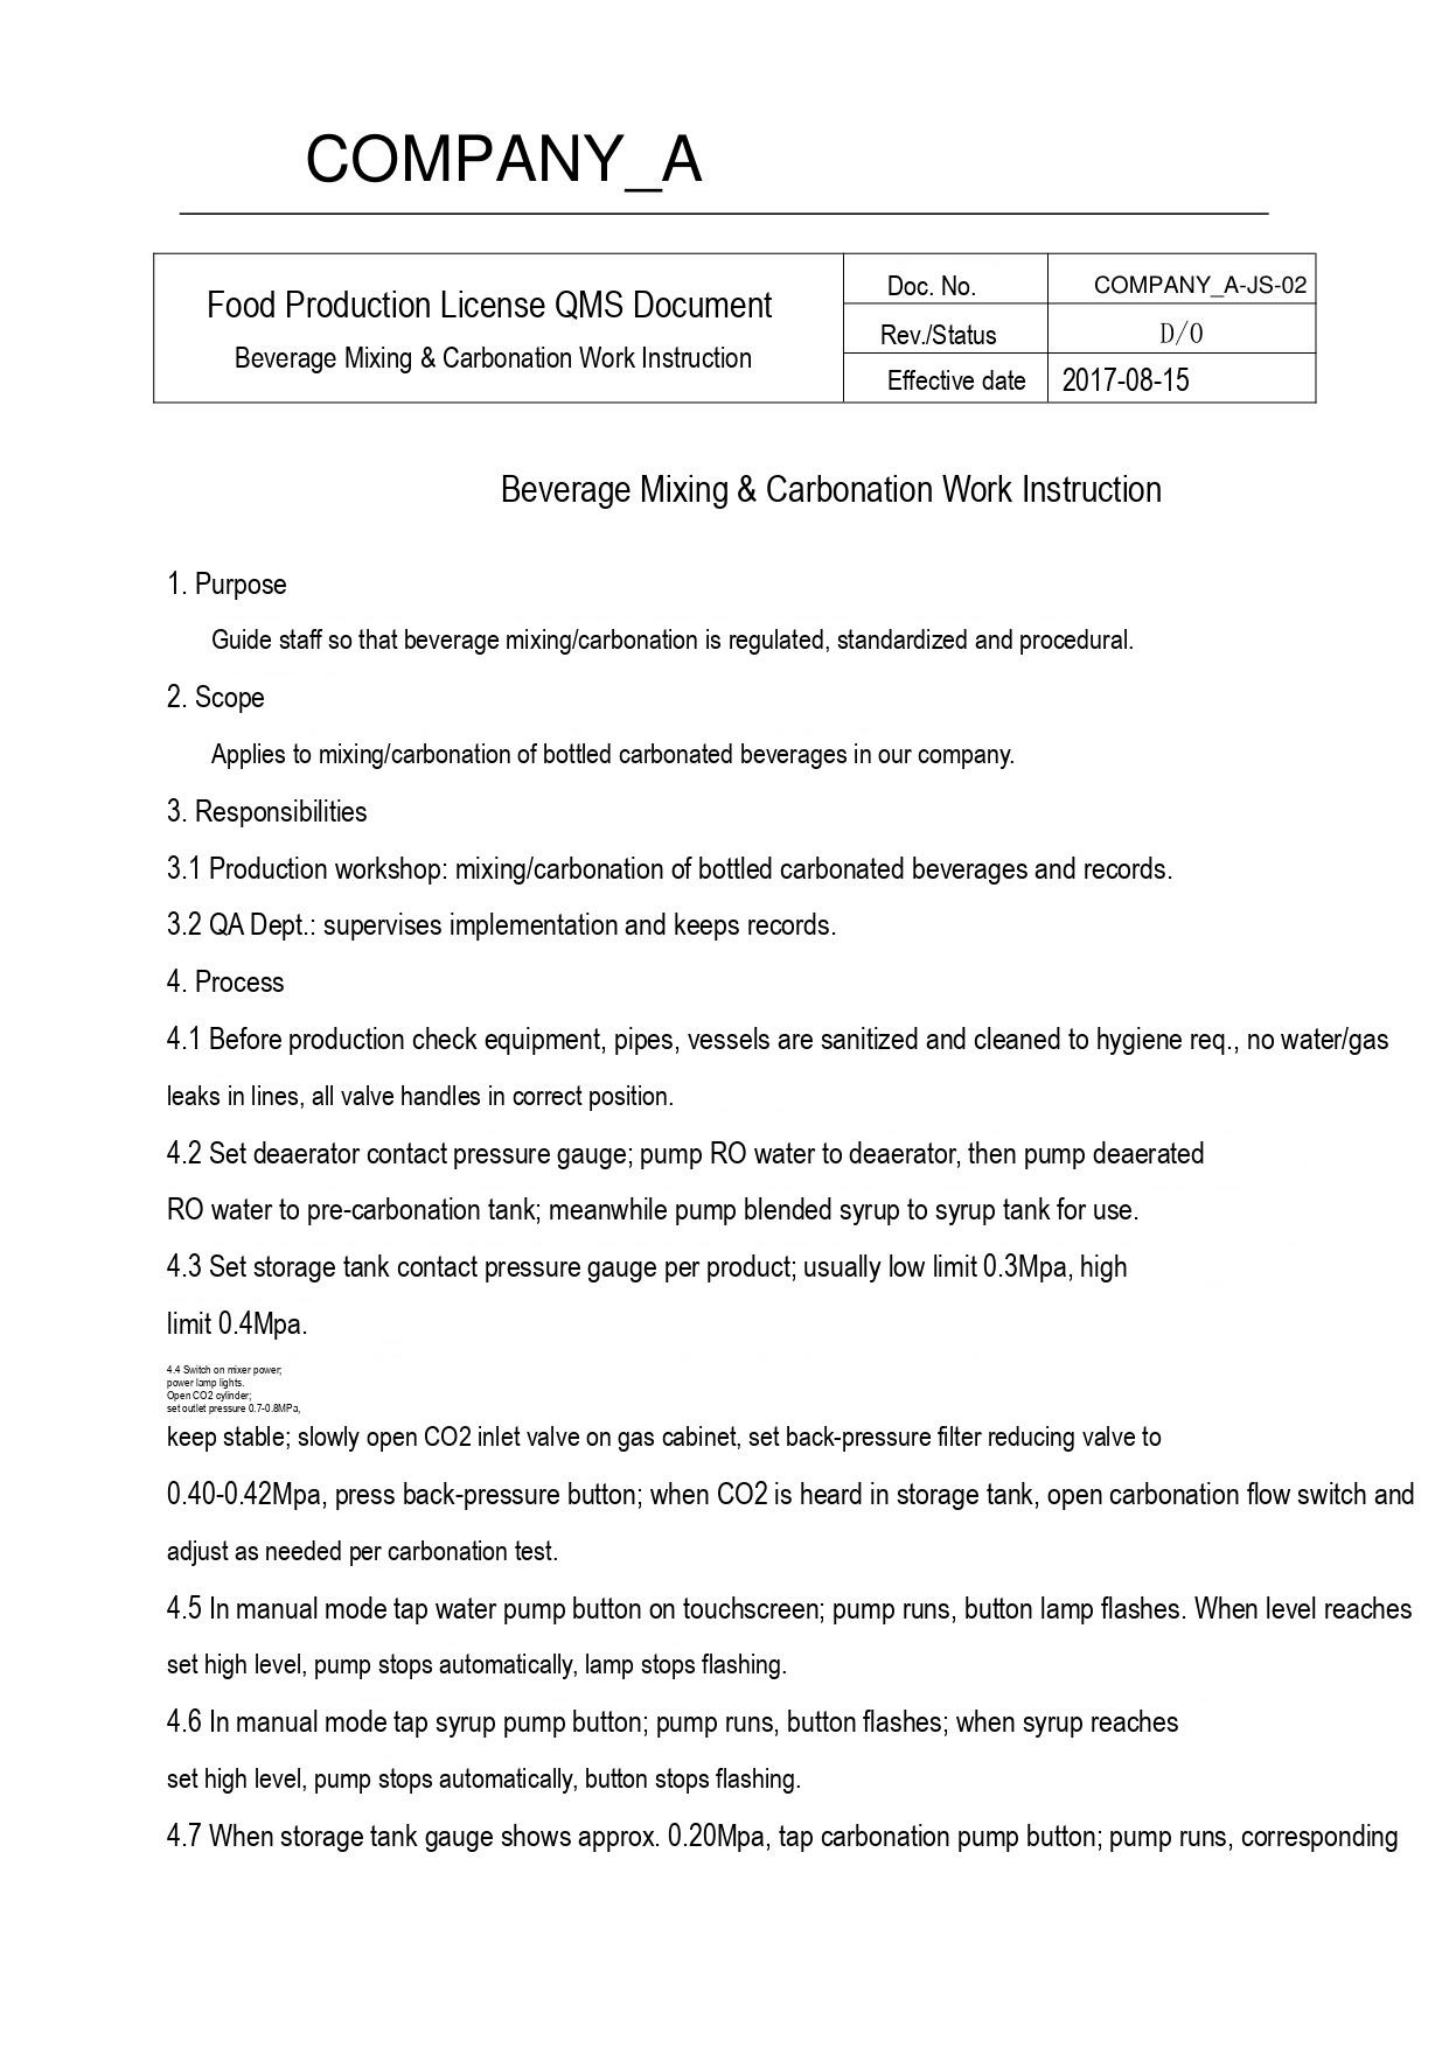COMPANY_A

| Food Production License QMS Document<br>Beverage Mixing & Carbonation Work Instruction | Doc. No. | COMPANY_A-JS-02 |
|---|---|---|
| | Rev./Status | D/0 |
| | Effective date | 2017-08-15 |

Beverage Mixing & Carbonation Work Instruction

1. Purpose

Guide staff so that beverage mixing/carbonation is regulated, standardized and procedural.

2. Scope

Applies to mixing/carbonation of bottled carbonated beverages in our company.

3. Responsibilities

3.1 Production workshop: mixing/carbonation of bottled carbonated beverages and records.

3.2 QA Dept.: supervises implementation and keeps records.

4. Process

4.1 Before production check equipment, pipes, vessels are sanitized and cleaned to hygiene req., no water/gas leaks in lines, all valve handles in correct position.

4.2 Set deaerator contact pressure gauge; pump RO water to deaerator, then pump deaerated RO water to pre-carbonation tank; meanwhile pump blended syrup to syrup tank for use.

4.3 Set storage tank contact pressure gauge per product; usually low limit 0.3Mpa, high limit 0.4Mpa.

4.4 Switch on mixer power; power lamp lights. Open CO2 cylinder; set outlet pressure 0.7-0.8MPa, keep stable; slowly open CO2 inlet valve on gas cabinet, set back-pressure filter reducing valve to 0.40-0.42Mpa, press back-pressure button; when CO2 is heard in storage tank, open carbonation flow switch and adjust as needed per carbonation test.

4.5 In manual mode tap water pump button on touchscreen; pump runs, button lamp flashes. When level reaches set high level, pump stops automatically, lamp stops flashing.

4.6 In manual mode tap syrup pump button; pump runs, button flashes; when syrup reaches set high level, pump stops automatically, button stops flashing.

4.7 When storage tank gauge shows approx. 0.20Mpa, tap carbonation pump button; pump runs, corresponding
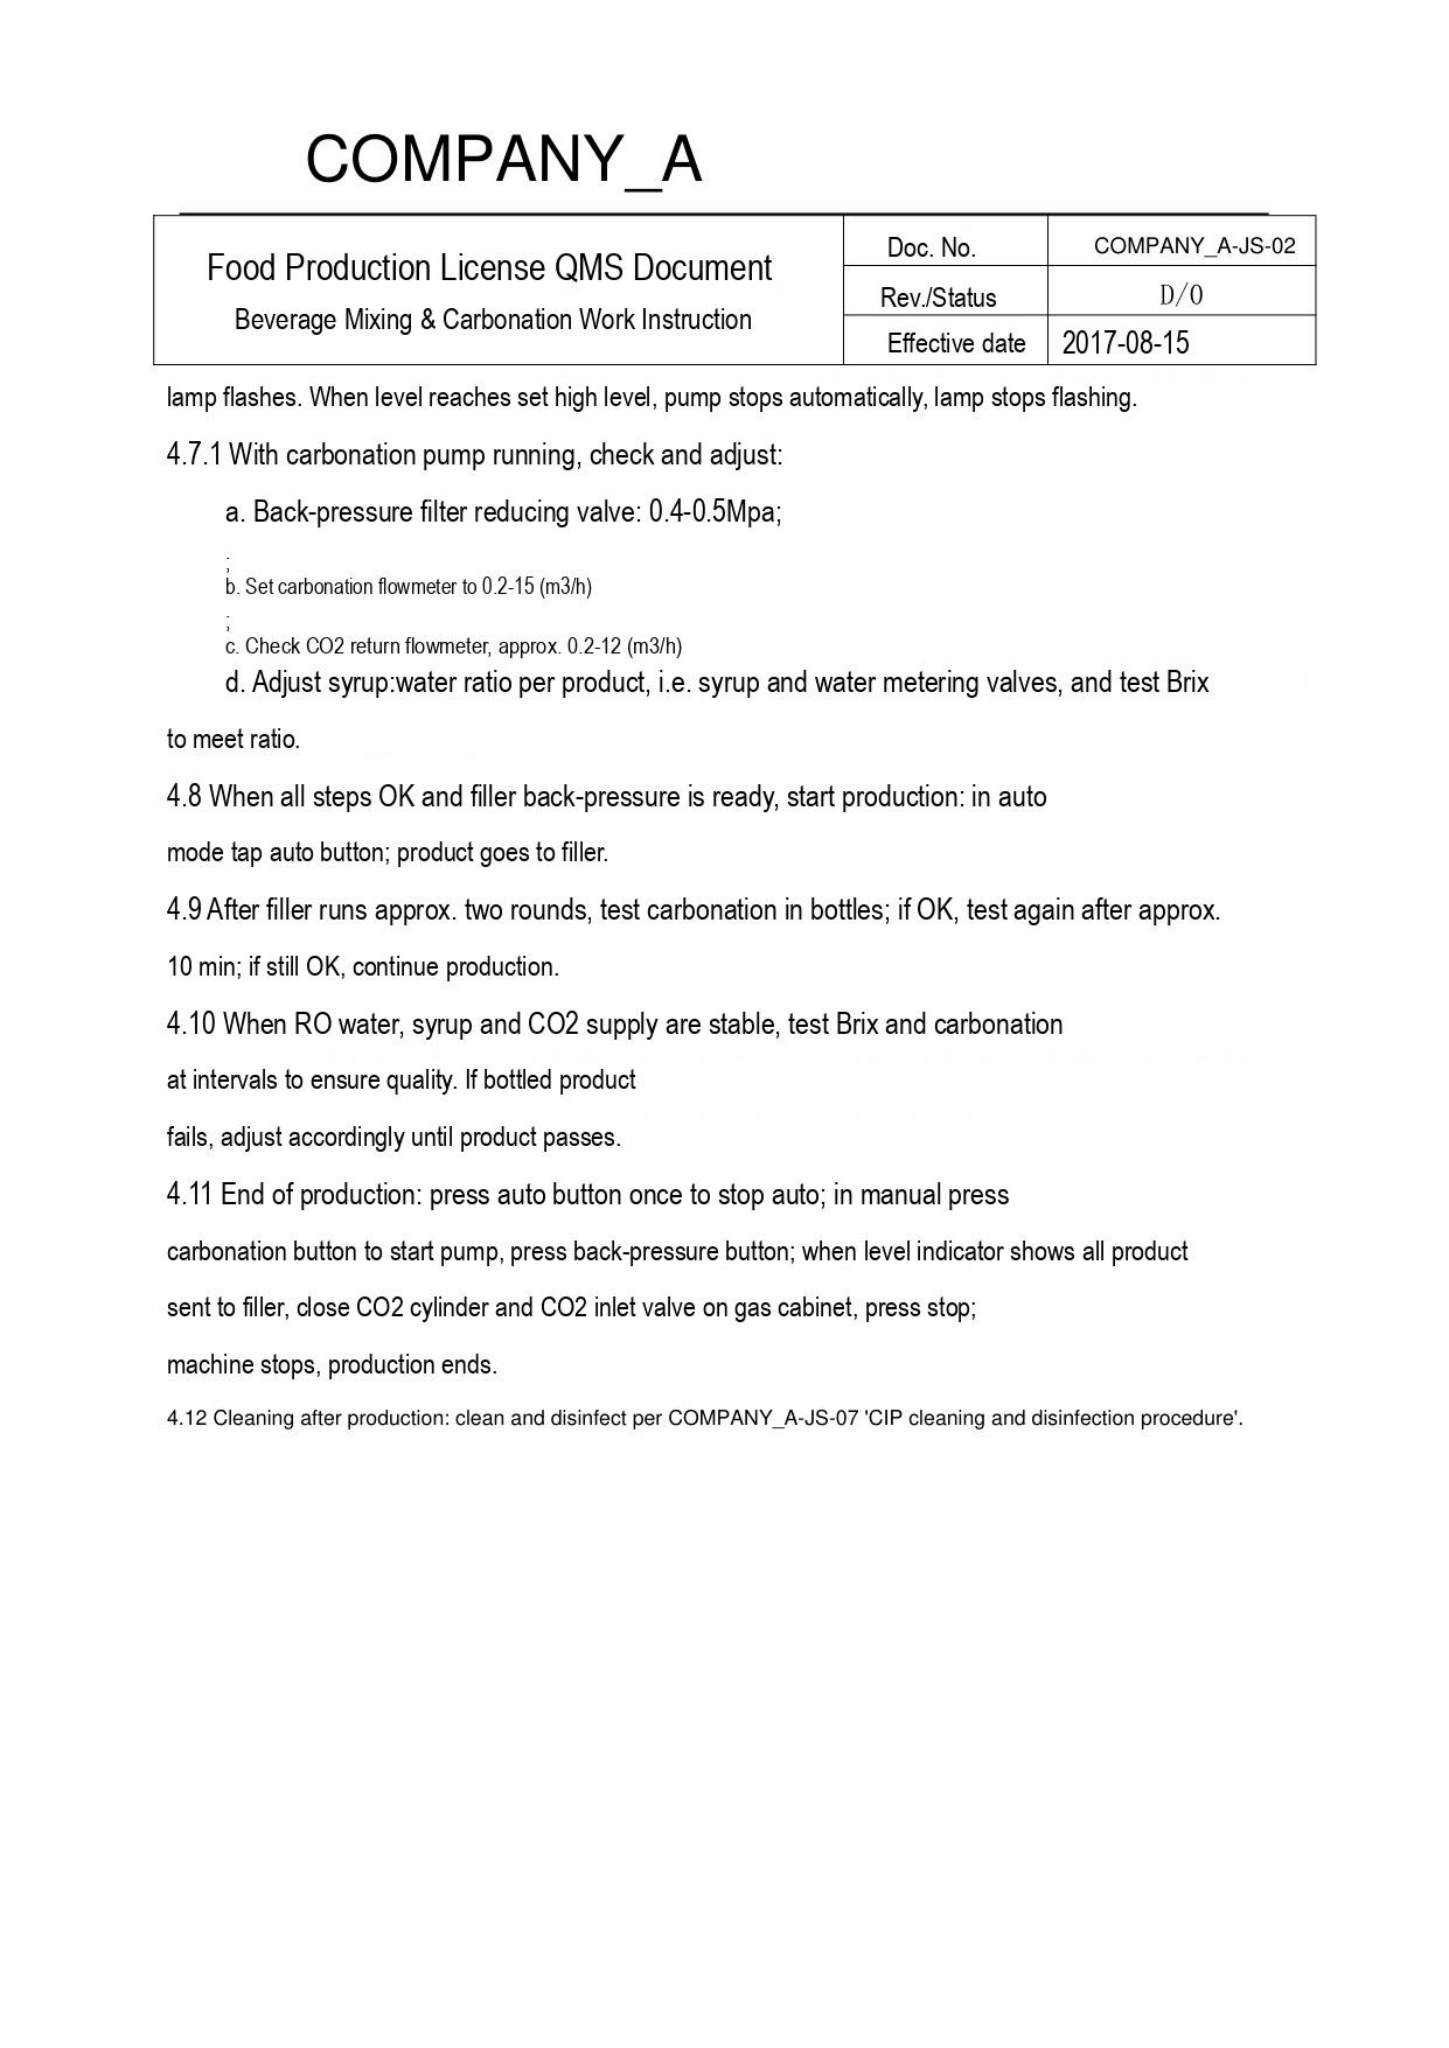COMPANY_A

| Food Production License QMS Document<br>Beverage Mixing & Carbonation Work Instruction | Doc. No. | COMPANY_A-JS-02 |
|---|---|---|
| | Rev./Status | D/0 |
| | Effective date | 2017-08-15 |

lamp flashes. When level reaches set high level, pump stops automatically, lamp stops flashing.

4.7.1 With carbonation pump running, check and adjust:

a. Back-pressure filter reducing valve: 0.4-0.5Mpa;

;
b. Set carbonation flowmeter to 0.2-15 (m3/h)

;
c. Check CO2 return flowmeter, approx. 0.2-12 (m3/h)

d. Adjust syrup:water ratio per product, i.e. syrup and water metering valves, and test Brix to meet ratio.

4.8 When all steps OK and filler back-pressure is ready, start production: in auto mode tap auto button; product goes to filler.

4.9 After filler runs approx. two rounds, test carbonation in bottles; if OK, test again after approx. 10 min; if still OK, continue production.

4.10 When RO water, syrup and CO2 supply are stable, test Brix and carbonation at intervals to ensure quality. If bottled product fails, adjust accordingly until product passes.

4.11 End of production: press auto button once to stop auto; in manual press carbonation button to start pump, press back-pressure button; when level indicator shows all product sent to filler, close CO2 cylinder and CO2 inlet valve on gas cabinet, press stop; machine stops, production ends.

4.12 Cleaning after production: clean and disinfect per COMPANY_A-JS-07 'CIP cleaning and disinfection procedure'.
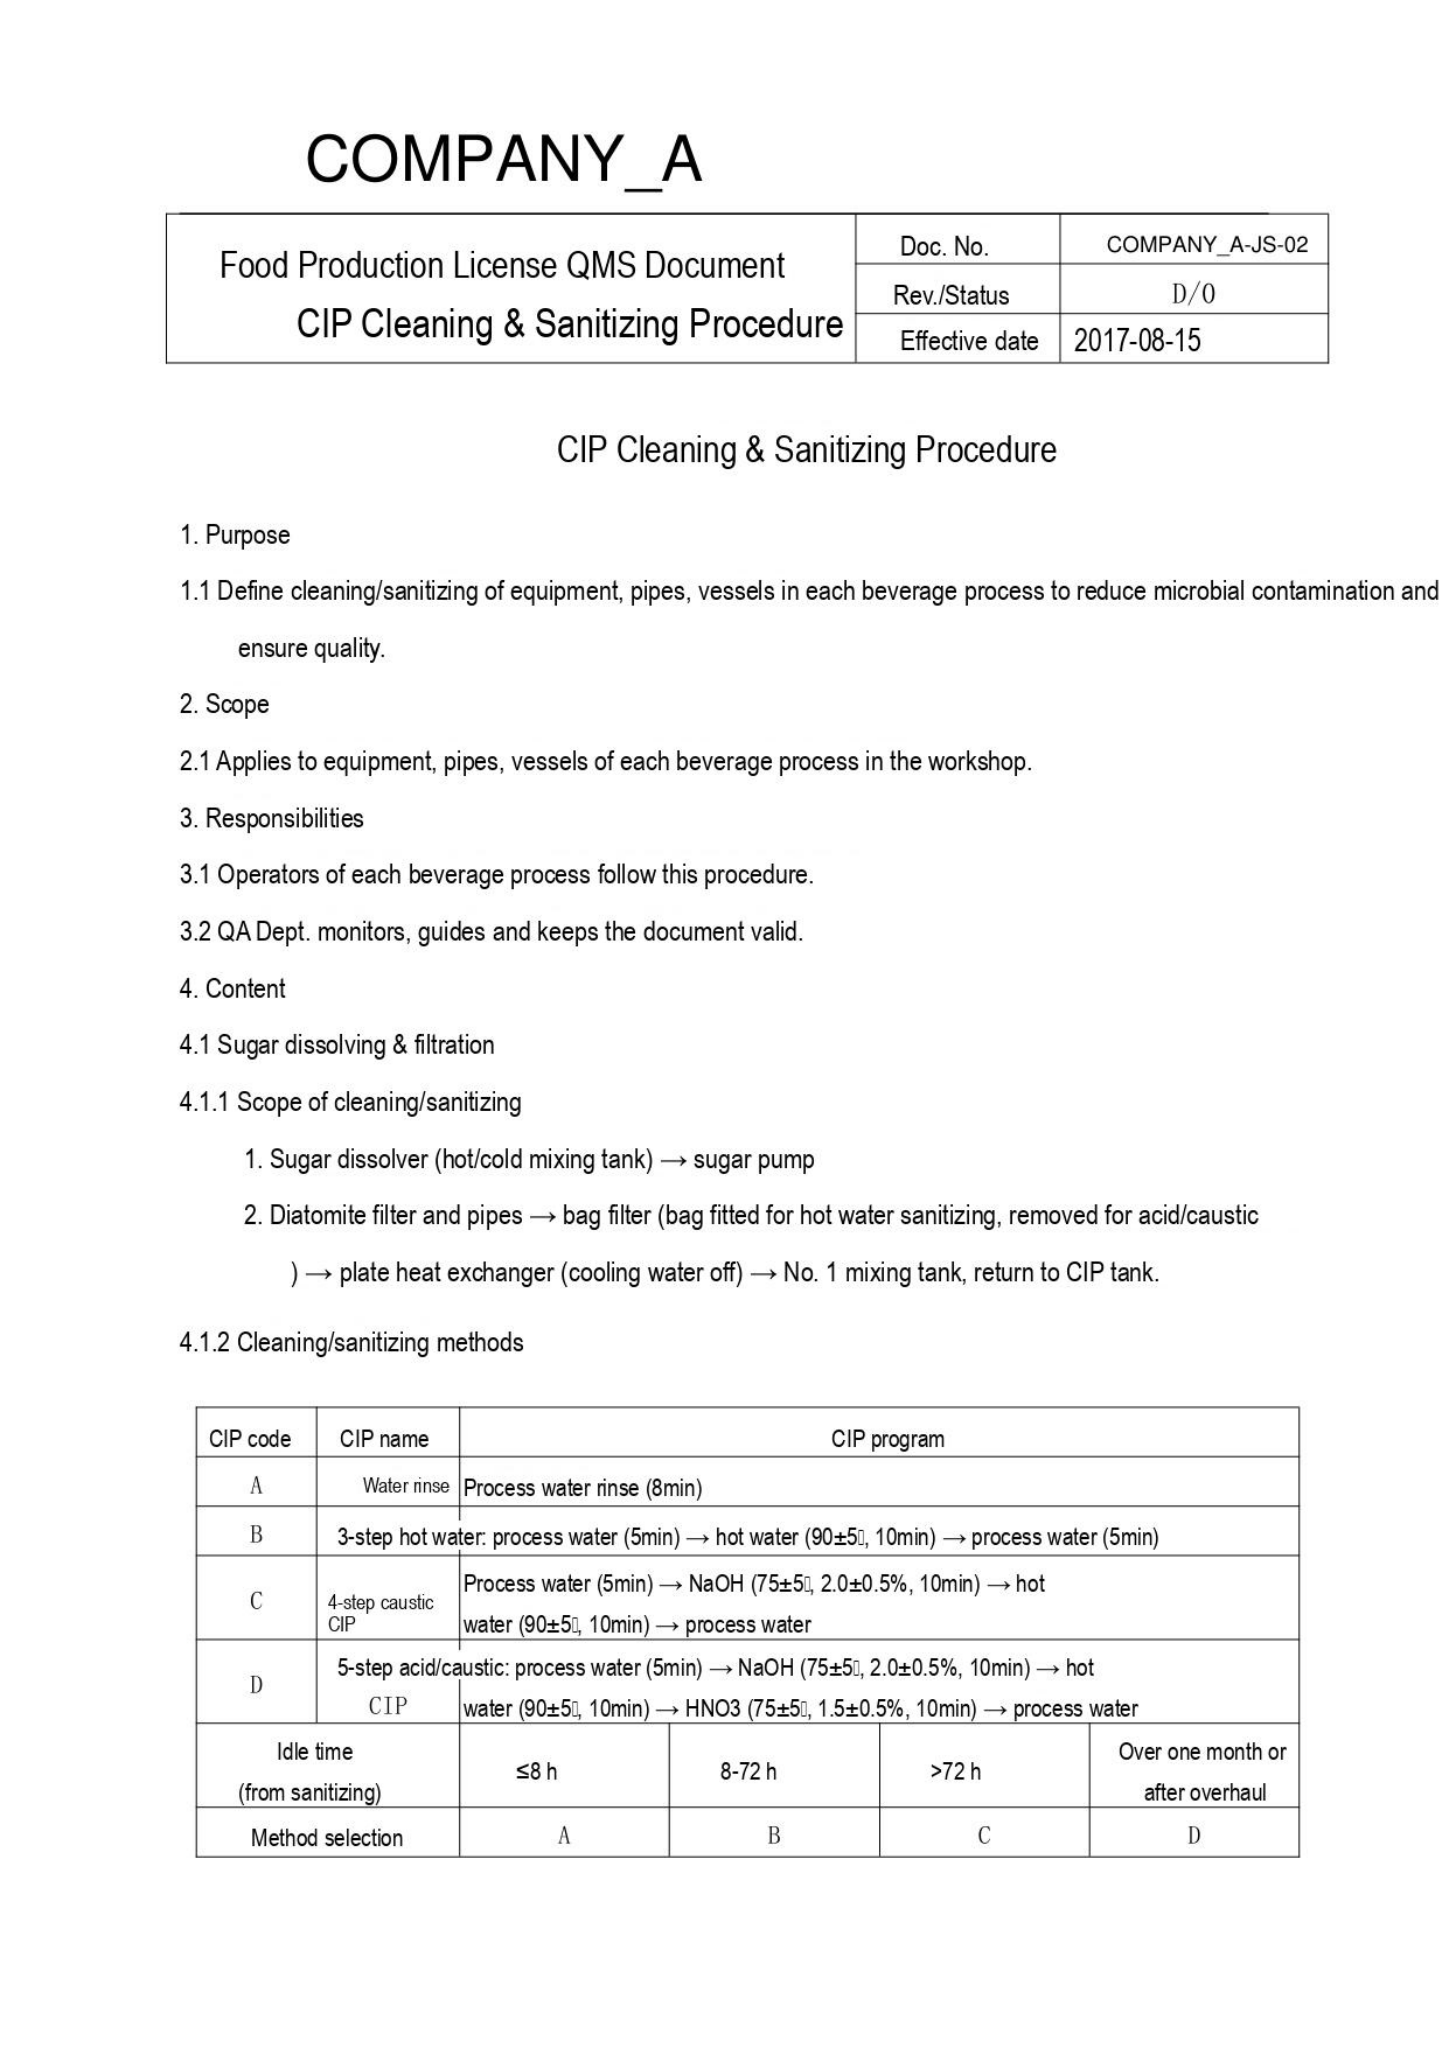# COMPANY_A

| Food Production License QMS Document CIP Cleaning & Sanitizing Procedure | Doc. No. | COMPANY_A-JS-02 |
|---|---|---|
| | Rev./Status | D/0 |
| | Effective date | 2017-08-15 |

CIP Cleaning & Sanitizing Procedure

1. Purpose

1.1 Define cleaning/sanitizing of equipment, pipes, vessels in each beverage process to reduce microbial contamination and ensure quality.

2. Scope

2.1 Applies to equipment, pipes, vessels of each beverage process in the workshop.

3. Responsibilities

3.1 Operators of each beverage process follow this procedure.

3.2 QA Dept. monitors, guides and keeps the document valid.

4. Content

4.1 Sugar dissolving & filtration

4.1.1 Scope of cleaning/sanitizing

1. Sugar dissolver (hot/cold mixing tank) → sugar pump

2. Diatomite filter and pipes → bag filter (bag fitted for hot water sanitizing, removed for acid/caustic ) → plate heat exchanger (cooling water off) → No. 1 mixing tank, return to CIP tank.

4.1.2 Cleaning/sanitizing methods

| CIP code | CIP name | CIP program |
|---|---|---|
| A | Water rinse | Process water rinse (8min) |
| B | 3-step hot water: | process water (5min) → hot water (90±5, 10min) → process water (5min) |
| C | 4-step caustic CIP | Process water (5min) → NaOH (75±5, 2.0±0.5%, 10min) → hot water (90±5, 10min) → process water |
| D | 5-step acid/caustic: CIP | process water (5min) → NaOH (75±5, 2.0±0.5%, 10min) → hot water (90±5, 10min) → HNO3 (75±5, 1.5±0.5%, 10min) → process water |

| Idle time (from sanitizing) | ≤8 h | 8-72 h | >72 h | Over one month or after overhaul |
|---|---|---|---|---|
| Method selection | A | B | C | D |
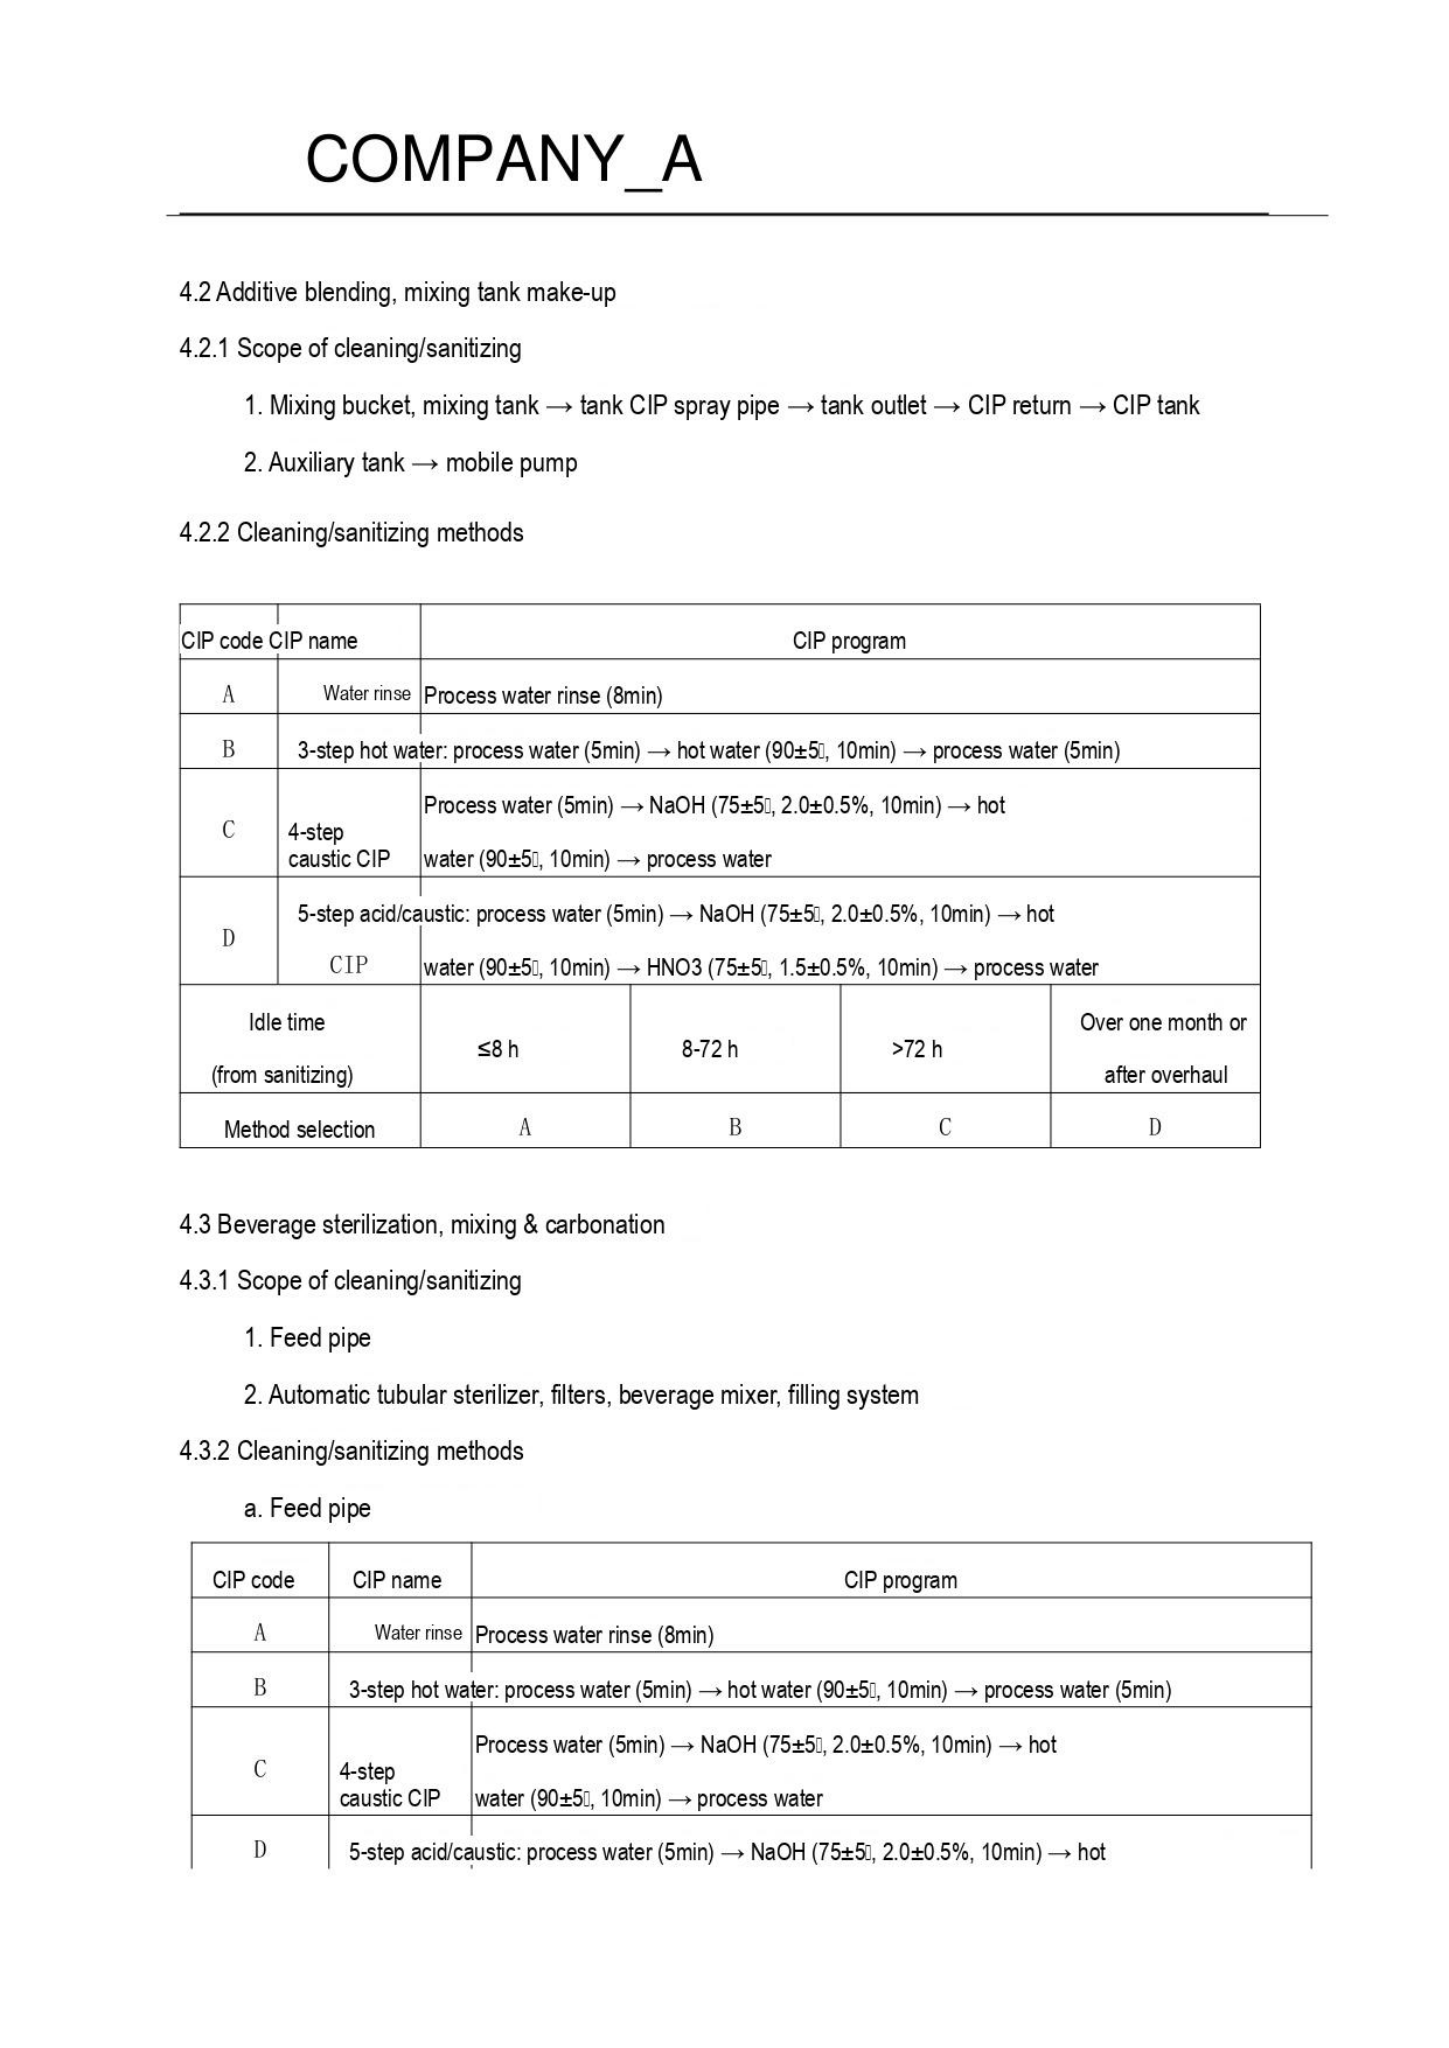COMPANY_A

4.2 Additive blending, mixing tank make-up

4.2.1 Scope of cleaning/sanitizing

1. Mixing bucket, mixing tank → tank CIP spray pipe → tank outlet → CIP return → CIP tank

2. Auxiliary tank → mobile pump

4.2.2 Cleaning/sanitizing methods

| CIP code | CIP name | CIP program | | | |
|---|---|---|---|---|---|
| A | Water rinse | Process water rinse (8min) | | | |
| B | 3-step hot water: | process water (5min) → hot water (90±5□, 10min) → process water (5min) | | | |
| C | 4-step caustic CIP | Process water (5min) → NaOH (75±5□, 2.0±0.5%, 10min) → hot water (90±5□, 10min) → process water | | | |
| D | 5-step acid/caustic: CIP | process water (5min) → NaOH (75±5□, 2.0±0.5%, 10min) → hot water (90±5□, 10min) → HNO3 (75±5□, 1.5±0.5%, 10min) → process water | | | |
| Idle time (from sanitizing) | | ≤8 h | 8-72 h | >72 h | Over one month or after overhaul |
| Method selection | | A | B | C | D |

4.3 Beverage sterilization, mixing & carbonation

4.3.1 Scope of cleaning/sanitizing

1. Feed pipe

2. Automatic tubular sterilizer, filters, beverage mixer, filling system

4.3.2 Cleaning/sanitizing methods

a. Feed pipe

| CIP code | CIP name | CIP program |
|---|---|---|
| A | Water rinse | Process water rinse (8min) |
| B | 3-step hot water: | process water (5min) → hot water (90±5□, 10min) → process water (5min) |
| C | 4-step caustic CIP | Process water (5min) → NaOH (75±5□, 2.0±0.5%, 10min) → hot water (90±5□, 10min) → process water |
| D | 5-step acid/caustic: | process water (5min) → NaOH (75±5□, 2.0±0.5%, 10min) → hot |
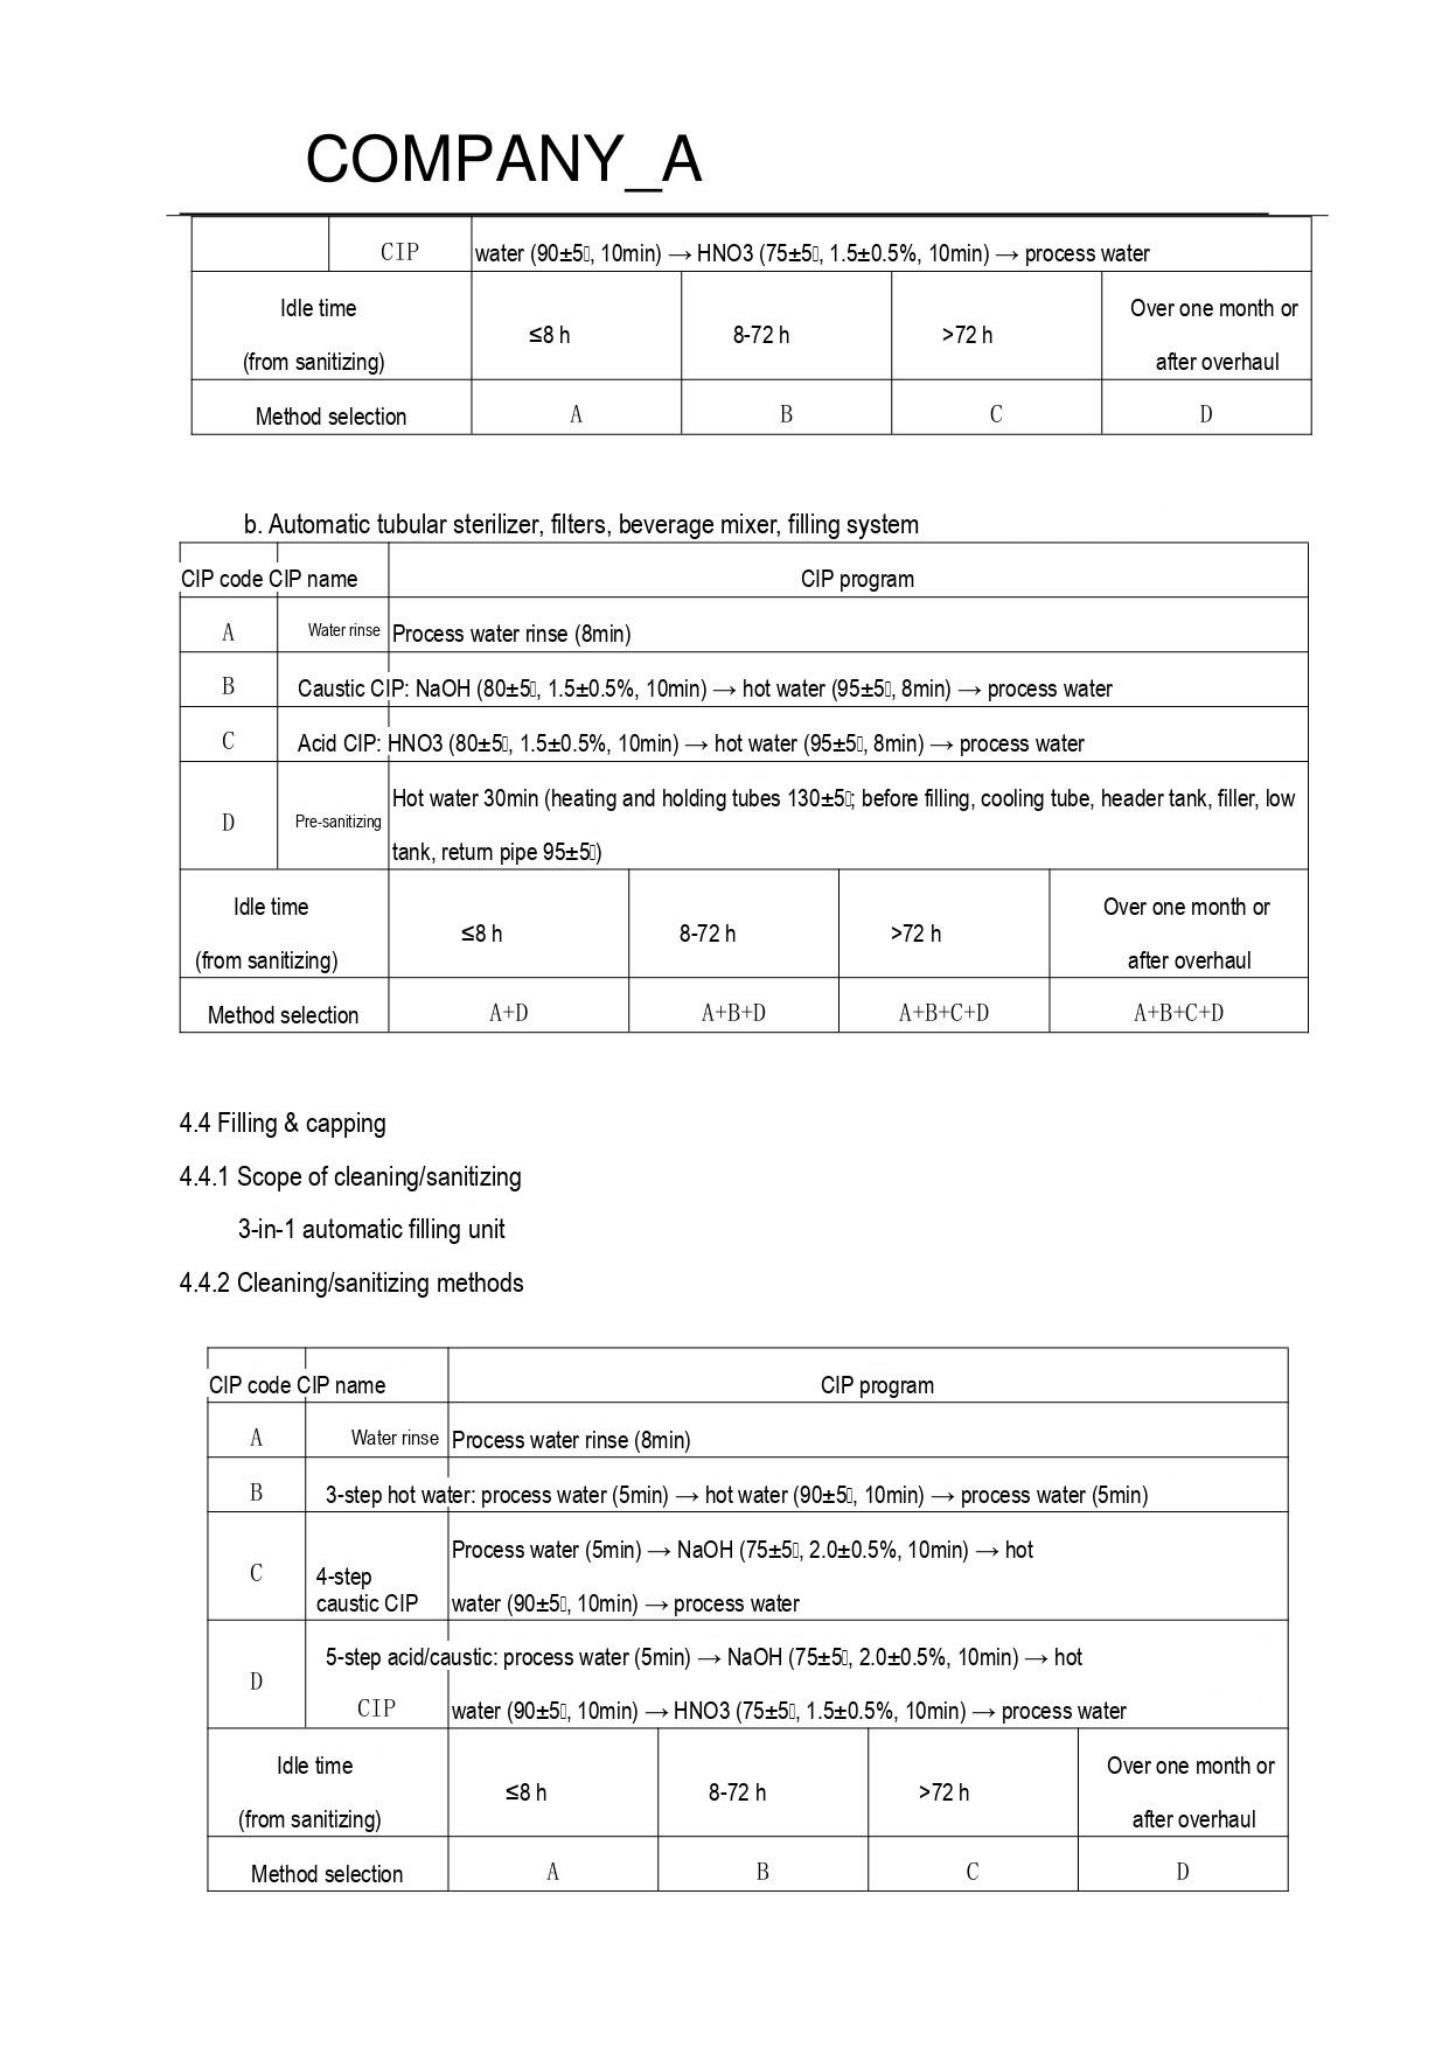COMPANY_A

|  | CIP | water (90±5□, 10min) → HNO3 (75±5□, 1.5±0.5%, 10min) → process water |  |  |
|---|---|---|---|---|
| Idle time (from sanitizing) |  | ≤8 h | 8-72 h | >72 h | Over one month or after overhaul |
| Method selection |  | A | B | C | D |

b. Automatic tubular sterilizer, filters, beverage mixer, filling system

| CIP code | CIP name | CIP program |  |  |  |
|---|---|---|---|---|---|
| A | Water rinse | Process water rinse (8min) |  |  |  |
| B | Caustic CIP: NaOH (80±5□, 1.5±0.5%, 10min) → hot water (95±5□, 8min) → process water |  |  |  |  |
| C | Acid CIP: HNO3 (80±5□, 1.5±0.5%, 10min) → hot water (95±5□, 8min) → process water |  |  |  |  |
| D | Pre-sanitizing | Hot water 30min (heating and holding tubes 130±5□; before filling, cooling tube, header tank, filler, low tank, return pipe 95±5□) |  |  |  |
| Idle time (from sanitizing) |  | ≤8 h | 8-72 h | >72 h | Over one month or after overhaul |
| Method selection |  | A+D | A+B+D | A+B+C+D | A+B+C+D |

4.4 Filling & capping

4.4.1 Scope of cleaning/sanitizing

3-in-1 automatic filling unit

4.4.2 Cleaning/sanitizing methods

| CIP code | CIP name | CIP program |  |  |  |
|---|---|---|---|---|---|
| A | Water rinse | Process water rinse (8min) |  |  |  |
| B | 3-step hot water: process water (5min) → hot water (90±5□, 10min) → process water (5min) |  |  |  |  |
| C | 4-step caustic CIP | Process water (5min) → NaOH (75±5□, 2.0±0.5%, 10min) → hot water (90±5□, 10min) → process water |  |  |  |
| D | 5-step acid/caustic: process water (5min) → NaOH (75±5□, 2.0±0.5%, 10min) → hot CIP water (90±5□, 10min) → HNO3 (75±5□, 1.5±0.5%, 10min) → process water |  |  |  |  |
| Idle time (from sanitizing) |  | ≤8 h | 8-72 h | >72 h | Over one month or after overhaul |
| Method selection |  | A | B | C | D |
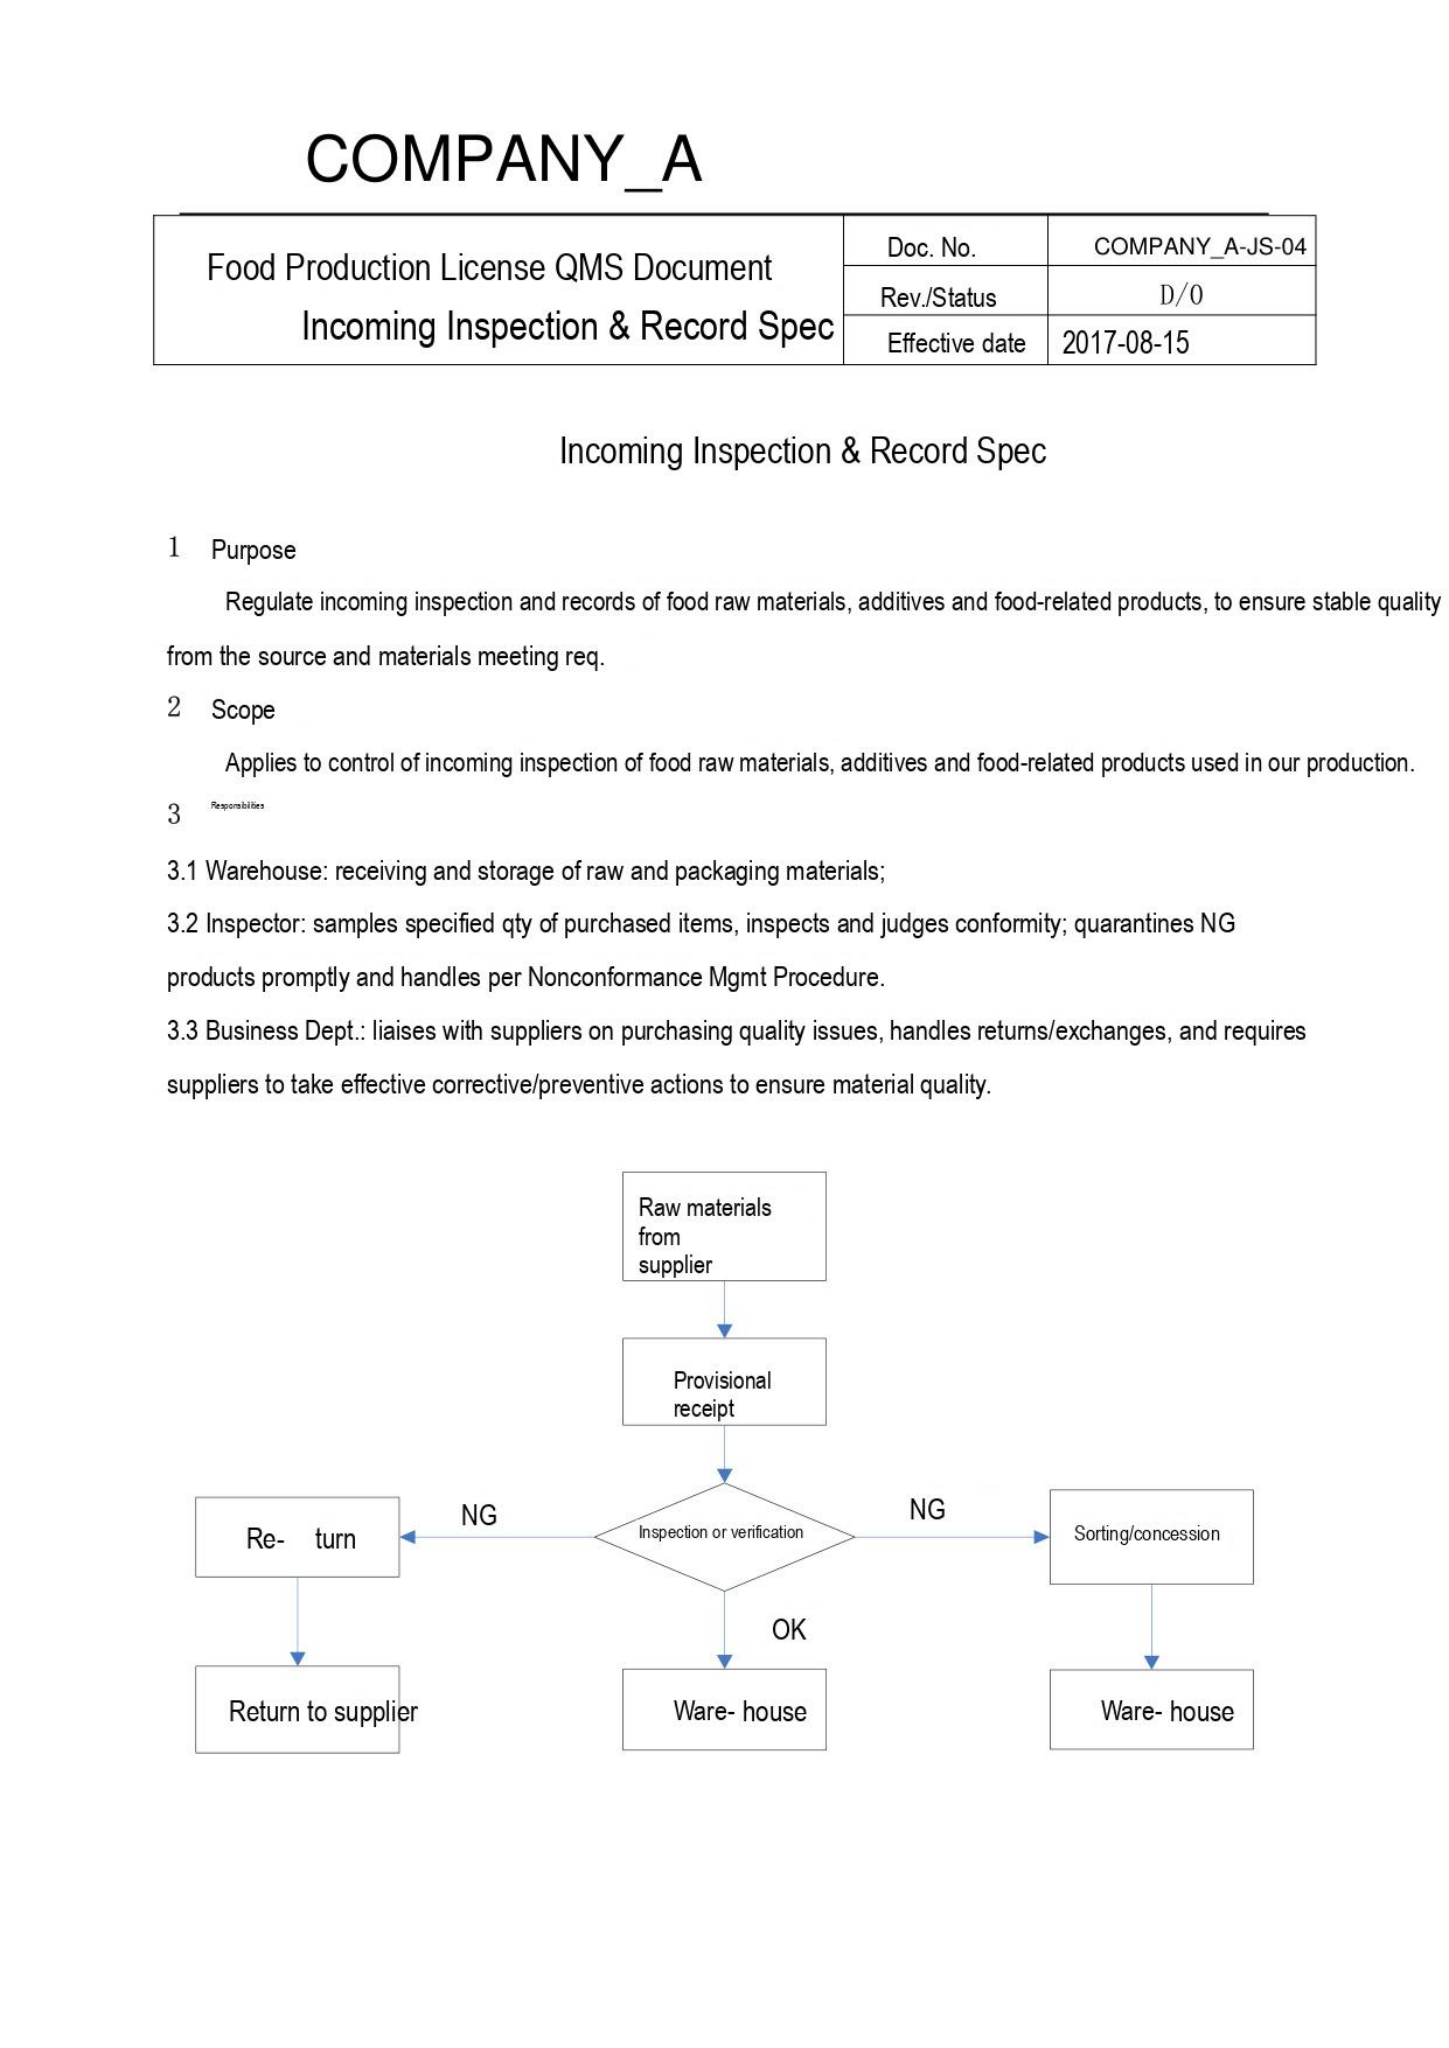COMPANY_A

| Food Production License QMS Document<br>Incoming Inspection & Record Spec | Doc. No. | COMPANY_A-JS-04 |
|---|---|---|
| | Rev./Status | D/0 |
| | Effective date | 2017-08-15 |

Incoming Inspection & Record Spec

1 Purpose

Regulate incoming inspection and records of food raw materials, additives and food-related products, to ensure stable quality from the source and materials meeting req.

2 Scope

Applies to control of incoming inspection of food raw materials, additives and food-related products used in our production.

3 Responsibilities

3.1 Warehouse: receiving and storage of raw and packaging materials;

3.2 Inspector: samples specified qty of purchased items, inspects and judges conformity; quarantines NG products promptly and handles per Nonconformance Mgmt Procedure.

3.3 Business Dept.: liaises with suppliers on purchasing quality issues, handles returns/exchanges, and requires suppliers to take effective corrective/preventive actions to ensure material quality.

Raw materials from supplier

Provisional receipt

Inspection or verification

NG

Re- turn

Return to supplier

OK

Ware- house

NG

Sorting/concession

Ware- house